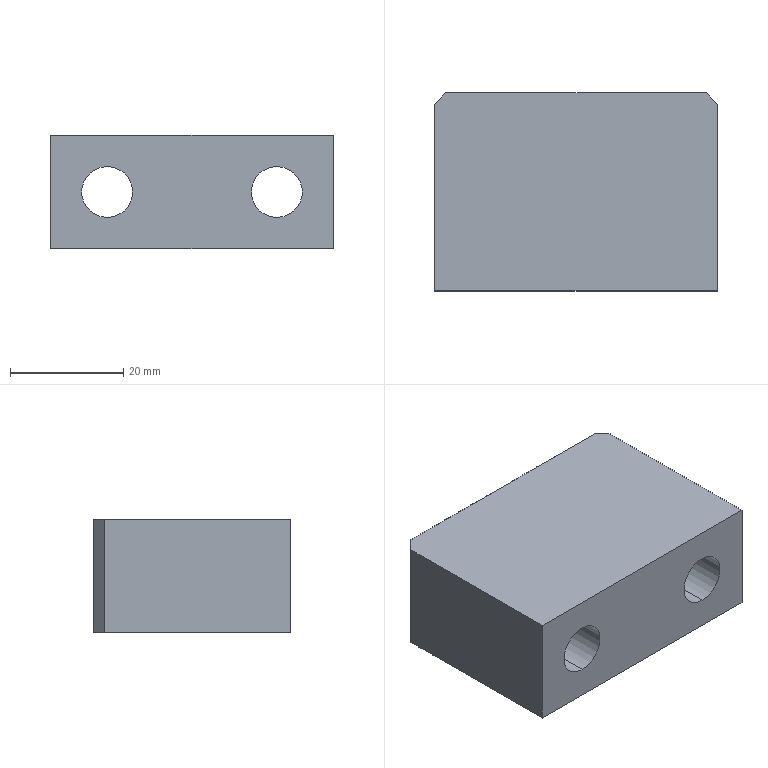Part | SolidWorks | features Chamfer 1, Extrusion 1, HoleWzd 1 | 1 solid | 18 faces | box 50 x 35 x 20 mm | volume 27074 mm3 | plane 10 | cylinder 8 | commonest cylinder face diameters 9 x4 15 x4
STEP:
#1=CARTESIAN_POINT('',(15.,2.5,-7.5));
#2=VERTEX_POINT('',#1);
#3=CARTESIAN_POINT('',(15.,2.5,7.5));
#4=VERTEX_POINT('',#3);
#5=CARTESIAN_POINT('',(15.,2.5,0.));
#6=DIRECTION('',(0.,1.,0.));
#7=DIRECTION('',(0.,0.,1.));
#8=AXIS2_PLACEMENT_3D('',#5,#6,#7);
#9=CIRCLE('',#8,7.5);
#10=EDGE_CURVE('',#2,#4,#9,.T.);
#11=ORIENTED_EDGE('',*,*,#10,.F.);
#12=CARTESIAN_POINT('',(15.,17.5,-7.5));
#13=VERTEX_POINT('',#12);
#14=CARTESIAN_POINT('',(15.,17.5,-7.5));
#15=DIRECTION('',(0.,1.,0.));
#16=VECTOR('',#15,1000.);
#17=LINE('',#14,#16);
#18=EDGE_CURVE('',#2,#13,#17,.T.);
#19=ORIENTED_EDGE('',*,*,#18,.T.);
#20=CARTESIAN_POINT('',(15.,17.5,7.5));
#21=VERTEX_POINT('',#20);
#22=CARTESIAN_POINT('',(15.,17.5,0.));
#23=DIRECTION('',(0.,1.,0.));
#24=DIRECTION('',(0.,0.,1.));
#25=AXIS2_PLACEMENT_3D('',#22,#23,#24);
#26=CIRCLE('',#25,7.5);
#27=EDGE_CURVE('',#13,#21,#26,.T.);
#28=ORIENTED_EDGE('',*,*,#27,.T.);
#29=CARTESIAN_POINT('',(15.,17.5,7.5));
#30=DIRECTION('',(0.,1.,0.));
#31=VECTOR('',#30,1000.);
#32=LINE('',#29,#31);
#33=EDGE_CURVE('',#4,#21,#32,.T.);
#34=ORIENTED_EDGE('',*,*,#33,.F.);
#35=EDGE_LOOP('',(#11,#19,#28,#34));
#36=FACE_OUTER_BOUND('',#35,.T.);
#37=CARTESIAN_POINT('',(15.,17.5,0.));
#38=DIRECTION('',(0.,1.,0.));
#39=DIRECTION('',(0.,0.,1.));
#40=AXIS2_PLACEMENT_3D('',#37,#38,#39);
#41=CYLINDRICAL_SURFACE('',#40,7.5);
#42=ADVANCED_FACE('',(#36),#41,.F.);
#43=CARTESIAN_POINT('',(15.,-17.5,-4.5));
#44=VERTEX_POINT('',#43);
#45=CARTESIAN_POINT('',(15.,-17.5,4.5));
#46=VERTEX_POINT('',#45);
#47=CARTESIAN_POINT('',(15.,-17.5,0.));
#48=DIRECTION('',(0.,1.,0.));
#49=DIRECTION('',(0.,0.,1.));
#50=AXIS2_PLACEMENT_3D('',#47,#48,#49);
#51=CIRCLE('',#50,4.5);
#52=EDGE_CURVE('',#44,#46,#51,.T.);
#53=ORIENTED_EDGE('',*,*,#52,.F.);
#54=CARTESIAN_POINT('',(15.,2.5,-4.5));
#55=VERTEX_POINT('',#54);
#56=CARTESIAN_POINT('',(15.,17.5,-4.5));
#57=DIRECTION('',(0.,1.,0.));
#58=VECTOR('',#57,1000.);
#59=LINE('',#56,#58);
#60=EDGE_CURVE('',#44,#55,#59,.T.);
#61=ORIENTED_EDGE('',*,*,#60,.T.);
#62=CARTESIAN_POINT('',(15.,2.5,4.5));
#63=VERTEX_POINT('',#62);
#64=CARTESIAN_POINT('',(15.,2.5,0.));
#65=DIRECTION('',(0.,1.,0.));
#66=DIRECTION('',(0.,0.,1.));
#67=AXIS2_PLACEMENT_3D('',#64,#65,#66);
#68=CIRCLE('',#67,4.5);
#69=EDGE_CURVE('',#55,#63,#68,.T.);
#70=ORIENTED_EDGE('',*,*,#69,.T.);
#71=CARTESIAN_POINT('',(15.,17.5,4.5));
#72=DIRECTION('',(0.,1.,0.));
#73=VECTOR('',#72,1000.);
#74=LINE('',#71,#73);
#75=EDGE_CURVE('',#46,#63,#74,.T.);
#76=ORIENTED_EDGE('',*,*,#75,.F.);
#77=EDGE_LOOP('',(#53,#61,#70,#76));
#78=FACE_OUTER_BOUND('',#77,.T.);
#79=CARTESIAN_POINT('',(15.,17.5,0.));
#80=DIRECTION('',(0.,1.,0.));
#81=DIRECTION('',(0.,0.,1.));
#82=AXIS2_PLACEMENT_3D('',#79,#80,#81);
#83=CYLINDRICAL_SURFACE('',#82,4.5);
#84=ADVANCED_FACE('',(#78),#83,.F.);
#85=CARTESIAN_POINT('',(-15.,2.5,-7.5));
#86=VERTEX_POINT('',#85);
#87=CARTESIAN_POINT('',(-15.,2.5,7.5));
#88=VERTEX_POINT('',#87);
#89=CARTESIAN_POINT('',(-15.,2.5,0.));
#90=DIRECTION('',(0.,1.,0.));
#91=DIRECTION('',(0.,0.,1.));
#92=AXIS2_PLACEMENT_3D('',#89,#90,#91);
#93=CIRCLE('',#92,7.5);
#94=EDGE_CURVE('',#86,#88,#93,.T.);
#95=ORIENTED_EDGE('',*,*,#94,.F.);
#96=CARTESIAN_POINT('',(-15.,17.5,-7.5));
#97=VERTEX_POINT('',#96);
#98=CARTESIAN_POINT('',(-15.,17.5,-7.5));
#99=DIRECTION('',(0.,1.,0.));
#100=VECTOR('',#99,1000.);
#101=LINE('',#98,#100);
#102=EDGE_CURVE('',#86,#97,#101,.T.);
#103=ORIENTED_EDGE('',*,*,#102,.T.);
#104=CARTESIAN_POINT('',(-15.,17.5,7.5));
#105=VERTEX_POINT('',#104);
#106=CARTESIAN_POINT('',(-15.,17.5,0.));
#107=DIRECTION('',(0.,1.,0.));
#108=DIRECTION('',(0.,0.,1.));
#109=AXIS2_PLACEMENT_3D('',#106,#107,#108);
#110=CIRCLE('',#109,7.5);
#111=EDGE_CURVE('',#97,#105,#110,.T.);
#112=ORIENTED_EDGE('',*,*,#111,.T.);
#113=CARTESIAN_POINT('',(-15.,17.5,7.5));
#114=DIRECTION('',(0.,1.,0.));
#115=VECTOR('',#114,1000.);
#116=LINE('',#113,#115);
#117=EDGE_CURVE('',#88,#105,#116,.T.);
#118=ORIENTED_EDGE('',*,*,#117,.F.);
#119=EDGE_LOOP('',(#95,#103,#112,#118));
#120=FACE_OUTER_BOUND('',#119,.T.);
#121=CARTESIAN_POINT('',(-15.,17.5,0.));
#122=DIRECTION('',(0.,1.,0.));
#123=DIRECTION('',(0.,0.,1.));
#124=AXIS2_PLACEMENT_3D('',#121,#122,#123);
#125=CYLINDRICAL_SURFACE('',#124,7.5);
#126=ADVANCED_FACE('',(#120),#125,.F.);
#127=CARTESIAN_POINT('',(-15.,-17.5,-4.5));
#128=VERTEX_POINT('',#127);
#129=CARTESIAN_POINT('',(-15.,-17.5,4.5));
#130=VERTEX_POINT('',#129);
#131=CARTESIAN_POINT('',(-15.,-17.5,0.));
#132=DIRECTION('',(0.,1.,0.));
#133=DIRECTION('',(0.,0.,1.));
#134=AXIS2_PLACEMENT_3D('',#131,#132,#133);
#135=CIRCLE('',#134,4.5);
#136=EDGE_CURVE('',#128,#130,#135,.T.);
#137=ORIENTED_EDGE('',*,*,#136,.F.);
#138=CARTESIAN_POINT('',(-15.,2.5,-4.5));
#139=VERTEX_POINT('',#138);
#140=CARTESIAN_POINT('',(-15.,17.5,-4.5));
#141=DIRECTION('',(0.,1.,0.));
#142=VECTOR('',#141,1000.);
#143=LINE('',#140,#142);
#144=EDGE_CURVE('',#128,#139,#143,.T.);
#145=ORIENTED_EDGE('',*,*,#144,.T.);
#146=CARTESIAN_POINT('',(-15.,2.5,4.5));
#147=VERTEX_POINT('',#146);
#148=CARTESIAN_POINT('',(-15.,2.5,0.));
#149=DIRECTION('',(0.,1.,0.));
#150=DIRECTION('',(0.,0.,1.));
#151=AXIS2_PLACEMENT_3D('',#148,#149,#150);
#152=CIRCLE('',#151,4.5);
#153=EDGE_CURVE('',#139,#147,#152,.T.);
#154=ORIENTED_EDGE('',*,*,#153,.T.);
#155=CARTESIAN_POINT('',(-15.,17.5,4.5));
#156=DIRECTION('',(0.,1.,0.));
#157=VECTOR('',#156,1000.);
#158=LINE('',#155,#157);
#159=EDGE_CURVE('',#130,#147,#158,.T.);
#160=ORIENTED_EDGE('',*,*,#159,.F.);
#161=EDGE_LOOP('',(#137,#145,#154,#160));
#162=FACE_OUTER_BOUND('',#161,.T.);
#163=CARTESIAN_POINT('',(-15.,17.5,0.));
#164=DIRECTION('',(0.,1.,0.));
#165=DIRECTION('',(0.,0.,1.));
#166=AXIS2_PLACEMENT_3D('',#163,#164,#165);
#167=CYLINDRICAL_SURFACE('',#166,4.5);
#168=ADVANCED_FACE('',(#162),#167,.F.);
#169=CARTESIAN_POINT('',(25.,-17.5,-10.));
#170=VERTEX_POINT('',#169);
#171=CARTESIAN_POINT('',(25.,15.5,-10.));
#172=VERTEX_POINT('',#171);
#173=CARTESIAN_POINT('',(25.,17.5,-10.));
#174=DIRECTION('',(0.,1.,0.));
#175=VECTOR('',#174,1000.);
#176=LINE('',#173,#175);
#177=EDGE_CURVE('',#170,#172,#176,.T.);
#178=ORIENTED_EDGE('',*,*,#177,.T.);
#179=CARTESIAN_POINT('',(25.,15.5,10.));
#180=VERTEX_POINT('',#179);
#181=CARTESIAN_POINT('',(25.,15.5,10.));
#182=DIRECTION('',(0.,0.,1.));
#183=VECTOR('',#182,1000.);
#184=LINE('',#181,#183);
#185=EDGE_CURVE('',#172,#180,#184,.T.);
#186=ORIENTED_EDGE('',*,*,#185,.T.);
#187=CARTESIAN_POINT('',(25.,-17.5,10.));
#188=VERTEX_POINT('',#187);
#189=CARTESIAN_POINT('',(25.,17.5,10.));
#190=DIRECTION('',(0.,1.,0.));
#191=VECTOR('',#190,1000.);
#192=LINE('',#189,#191);
#193=EDGE_CURVE('',#188,#180,#192,.T.);
#194=ORIENTED_EDGE('',*,*,#193,.F.);
#195=CARTESIAN_POINT('',(25.,-17.5,10.));
#196=DIRECTION('',(0.,0.,-1.));
#197=VECTOR('',#196,1000.);
#198=LINE('',#195,#197);
#199=EDGE_CURVE('',#188,#170,#198,.T.);
#200=ORIENTED_EDGE('',*,*,#199,.T.);
#201=EDGE_LOOP('',(#178,#186,#194,#200));
#202=FACE_OUTER_BOUND('',#201,.T.);
#203=CARTESIAN_POINT('',(25.,17.5,10.));
#204=DIRECTION('',(-1.,0.,0.));
#205=DIRECTION('',(0.,-1.,0.));
#206=AXIS2_PLACEMENT_3D('',#203,#204,#205);
#207=PLANE('',#206);
#208=ADVANCED_FACE('',(#202),#207,.F.);
#209=CARTESIAN_POINT('',(15.,17.5,0.));
#210=DIRECTION('',(0.,1.,0.));
#211=DIRECTION('',(0.,0.,1.));
#212=AXIS2_PLACEMENT_3D('',#209,#210,#211);
#213=CIRCLE('',#212,7.5);
#214=EDGE_CURVE('',#21,#13,#213,.T.);
#215=ORIENTED_EDGE('',*,*,#214,.F.);
#216=ORIENTED_EDGE('',*,*,#27,.F.);
#217=EDGE_LOOP('',(#215,#216));
#218=FACE_BOUND('',#217,.T.);
#219=CARTESIAN_POINT('',(-15.,17.5,0.));
#220=DIRECTION('',(0.,1.,0.));
#221=DIRECTION('',(0.,0.,1.));
#222=AXIS2_PLACEMENT_3D('',#219,#220,#221);
#223=CIRCLE('',#222,7.5);
#224=EDGE_CURVE('',#105,#97,#223,.T.);
#225=ORIENTED_EDGE('',*,*,#224,.F.);
#226=ORIENTED_EDGE('',*,*,#111,.F.);
#227=EDGE_LOOP('',(#225,#226));
#228=FACE_BOUND('',#227,.T.);
#229=CARTESIAN_POINT('',(23.,17.5,10.));
#230=VERTEX_POINT('',#229);
#231=CARTESIAN_POINT('',(-23.,17.5,10.));
#232=VERTEX_POINT('',#231);
#233=CARTESIAN_POINT('',(-25.,17.5,10.));
#234=DIRECTION('',(-1.,0.,0.));
#235=VECTOR('',#234,1000.);
#236=LINE('',#233,#235);
#237=EDGE_CURVE('',#230,#232,#236,.T.);
#238=ORIENTED_EDGE('',*,*,#237,.F.);
#239=CARTESIAN_POINT('',(23.,17.5,-10.));
#240=VERTEX_POINT('',#239);
#241=CARTESIAN_POINT('',(23.,17.5,10.));
#242=DIRECTION('',(0.,0.,-1.));
#243=VECTOR('',#242,1000.);
#244=LINE('',#241,#243);
#245=EDGE_CURVE('',#230,#240,#244,.T.);
#246=ORIENTED_EDGE('',*,*,#245,.T.);
#247=CARTESIAN_POINT('',(-23.,17.5,-10.));
#248=VERTEX_POINT('',#247);
#249=CARTESIAN_POINT('',(-25.,17.5,-10.));
#250=DIRECTION('',(-1.,0.,0.));
#251=VECTOR('',#250,1000.);
#252=LINE('',#249,#251);
#253=EDGE_CURVE('',#240,#248,#252,.T.);
#254=ORIENTED_EDGE('',*,*,#253,.T.);
#255=CARTESIAN_POINT('',(-23.,17.5,10.));
#256=DIRECTION('',(0.,0.,1.));
#257=VECTOR('',#256,1000.);
#258=LINE('',#255,#257);
#259=EDGE_CURVE('',#248,#232,#258,.T.);
#260=ORIENTED_EDGE('',*,*,#259,.T.);
#261=EDGE_LOOP('',(#238,#246,#254,#260));
#262=FACE_OUTER_BOUND('',#261,.T.);
#263=CARTESIAN_POINT('',(-25.,17.5,10.));
#264=DIRECTION('',(0.,-1.,0.));
#265=DIRECTION('',(0.,0.,-1.));
#266=AXIS2_PLACEMENT_3D('',#263,#264,#265);
#267=PLANE('',#266);
#268=ADVANCED_FACE('',(#218,#228,#262),#267,.F.);
#269=CARTESIAN_POINT('',(-25.,15.5,10.));
#270=VERTEX_POINT('',#269);
#271=CARTESIAN_POINT('',(-25.,-17.5,10.));
#272=VERTEX_POINT('',#271);
#273=CARTESIAN_POINT('',(-25.,17.5,10.));
#274=DIRECTION('',(0.,-1.,0.));
#275=VECTOR('',#274,1000.);
#276=LINE('',#273,#275);
#277=EDGE_CURVE('',#270,#272,#276,.T.);
#278=ORIENTED_EDGE('',*,*,#277,.F.);
#279=CARTESIAN_POINT('',(-25.,15.5,-10.));
#280=VERTEX_POINT('',#279);
#281=CARTESIAN_POINT('',(-25.,15.5,10.));
#282=DIRECTION('',(0.,0.,-1.));
#283=VECTOR('',#282,1000.);
#284=LINE('',#281,#283);
#285=EDGE_CURVE('',#270,#280,#284,.T.);
#286=ORIENTED_EDGE('',*,*,#285,.T.);
#287=CARTESIAN_POINT('',(-25.,-17.5,-10.));
#288=VERTEX_POINT('',#287);
#289=CARTESIAN_POINT('',(-25.,17.5,-10.));
#290=DIRECTION('',(0.,-1.,0.));
#291=VECTOR('',#290,1000.);
#292=LINE('',#289,#291);
#293=EDGE_CURVE('',#280,#288,#292,.T.);
#294=ORIENTED_EDGE('',*,*,#293,.T.);
#295=CARTESIAN_POINT('',(-25.,-17.5,10.));
#296=DIRECTION('',(0.,0.,-1.));
#297=VECTOR('',#296,1000.);
#298=LINE('',#295,#297);
#299=EDGE_CURVE('',#272,#288,#298,.T.);
#300=ORIENTED_EDGE('',*,*,#299,.F.);
#301=EDGE_LOOP('',(#278,#286,#294,#300));
#302=FACE_OUTER_BOUND('',#301,.T.);
#303=CARTESIAN_POINT('',(-25.,17.5,10.));
#304=DIRECTION('',(1.,0.,0.));
#305=DIRECTION('',(0.,1.,0.));
#306=AXIS2_PLACEMENT_3D('',#303,#304,#305);
#307=PLANE('',#306);
#308=ADVANCED_FACE('',(#302),#307,.F.);
#309=CARTESIAN_POINT('',(15.,-17.5,0.));
#310=DIRECTION('',(0.,1.,0.));
#311=DIRECTION('',(0.,0.,1.));
#312=AXIS2_PLACEMENT_3D('',#309,#310,#311);
#313=CIRCLE('',#312,4.5);
#314=EDGE_CURVE('',#46,#44,#313,.T.);
#315=ORIENTED_EDGE('',*,*,#314,.T.);
#316=ORIENTED_EDGE('',*,*,#52,.T.);
#317=EDGE_LOOP('',(#315,#316));
#318=FACE_BOUND('',#317,.T.);
#319=CARTESIAN_POINT('',(-15.,-17.5,0.));
#320=DIRECTION('',(0.,1.,0.));
#321=DIRECTION('',(0.,0.,1.));
#322=AXIS2_PLACEMENT_3D('',#319,#320,#321);
#323=CIRCLE('',#322,4.5);
#324=EDGE_CURVE('',#130,#128,#323,.T.);
#325=ORIENTED_EDGE('',*,*,#324,.T.);
#326=ORIENTED_EDGE('',*,*,#136,.T.);
#327=EDGE_LOOP('',(#325,#326));
#328=FACE_BOUND('',#327,.T.);
#329=CARTESIAN_POINT('',(-25.,-17.5,-10.));
#330=DIRECTION('',(1.,0.,0.));
#331=VECTOR('',#330,1000.);
#332=LINE('',#329,#331);
#333=EDGE_CURVE('',#288,#170,#332,.T.);
#334=ORIENTED_EDGE('',*,*,#333,.T.);
#335=ORIENTED_EDGE('',*,*,#199,.F.);
#336=CARTESIAN_POINT('',(-25.,-17.5,10.));
#337=DIRECTION('',(1.,0.,0.));
#338=VECTOR('',#337,1000.);
#339=LINE('',#336,#338);
#340=EDGE_CURVE('',#272,#188,#339,.T.);
#341=ORIENTED_EDGE('',*,*,#340,.F.);
#342=ORIENTED_EDGE('',*,*,#299,.T.);
#343=EDGE_LOOP('',(#334,#335,#341,#342));
#344=FACE_OUTER_BOUND('',#343,.T.);
#345=CARTESIAN_POINT('',(-25.,-17.5,10.));
#346=DIRECTION('',(0.,1.,0.));
#347=DIRECTION('',(0.,0.,1.));
#348=AXIS2_PLACEMENT_3D('',#345,#346,#347);
#349=PLANE('',#348);
#350=ADVANCED_FACE('',(#318,#328,#344),#349,.F.);
#351=ORIENTED_EDGE('',*,*,#193,.T.);
#352=CARTESIAN_POINT('',(20.25,20.25,10.));
#353=DIRECTION('',(-0.7071,0.7071,0.));
#354=VECTOR('',#353,1000.);
#355=LINE('',#352,#354);
#356=EDGE_CURVE('',#180,#230,#355,.T.);
#357=ORIENTED_EDGE('',*,*,#356,.T.);
#358=ORIENTED_EDGE('',*,*,#237,.T.);
#359=CARTESIAN_POINT('',(-20.25,20.25,10.));
#360=DIRECTION('',(-0.7071,-0.7071,0.));
#361=VECTOR('',#360,1000.);
#362=LINE('',#359,#361);
#363=EDGE_CURVE('',#232,#270,#362,.T.);
#364=ORIENTED_EDGE('',*,*,#363,.T.);
#365=ORIENTED_EDGE('',*,*,#277,.T.);
#366=ORIENTED_EDGE('',*,*,#340,.T.);
#367=EDGE_LOOP('',(#351,#357,#358,#364,#365,#366));
#368=FACE_OUTER_BOUND('',#367,.T.);
#369=CARTESIAN_POINT('',(0.,0.,10.));
#370=DIRECTION('',(0.,0.,1.));
#371=DIRECTION('',(1.,0.,0.));
#372=AXIS2_PLACEMENT_3D('',#369,#370,#371);
#373=PLANE('',#372);
#374=ADVANCED_FACE('',(#368),#373,.T.);
#375=ORIENTED_EDGE('',*,*,#253,.F.);
#376=CARTESIAN_POINT('',(23.,17.5,-10.));
#377=DIRECTION('',(0.7071,-0.7071,0.));
#378=VECTOR('',#377,1000.);
#379=LINE('',#376,#378);
#380=EDGE_CURVE('',#240,#172,#379,.T.);
#381=ORIENTED_EDGE('',*,*,#380,.T.);
#382=ORIENTED_EDGE('',*,*,#177,.F.);
#383=ORIENTED_EDGE('',*,*,#333,.F.);
#384=ORIENTED_EDGE('',*,*,#293,.F.);
#385=CARTESIAN_POINT('',(-25.,15.5,-10.));
#386=DIRECTION('',(0.7071,0.7071,0.));
#387=VECTOR('',#386,1000.);
#388=LINE('',#385,#387);
#389=EDGE_CURVE('',#280,#248,#388,.T.);
#390=ORIENTED_EDGE('',*,*,#389,.T.);
#391=EDGE_LOOP('',(#375,#381,#382,#383,#384,#390));
#392=FACE_OUTER_BOUND('',#391,.T.);
#393=CARTESIAN_POINT('',(0.,0.,-10.));
#394=DIRECTION('',(0.,0.,1.));
#395=DIRECTION('',(1.,0.,0.));
#396=AXIS2_PLACEMENT_3D('',#393,#394,#395);
#397=PLANE('',#396);
#398=ADVANCED_FACE('',(#392),#397,.F.);
#399=ORIENTED_EDGE('',*,*,#144,.F.);
#400=ORIENTED_EDGE('',*,*,#324,.F.);
#401=ORIENTED_EDGE('',*,*,#159,.T.);
#402=CARTESIAN_POINT('',(-15.,2.5,0.));
#403=DIRECTION('',(0.,1.,0.));
#404=DIRECTION('',(0.,0.,1.));
#405=AXIS2_PLACEMENT_3D('',#402,#403,#404);
#406=CIRCLE('',#405,4.5);
#407=EDGE_CURVE('',#147,#139,#406,.T.);
#408=ORIENTED_EDGE('',*,*,#407,.T.);
#409=EDGE_LOOP('',(#399,#400,#401,#408));
#410=FACE_OUTER_BOUND('',#409,.T.);
#411=CARTESIAN_POINT('',(-15.,17.5,0.));
#412=DIRECTION('',(0.,1.,0.));
#413=DIRECTION('',(0.,0.,1.));
#414=AXIS2_PLACEMENT_3D('',#411,#412,#413);
#415=CYLINDRICAL_SURFACE('',#414,4.5);
#416=ADVANCED_FACE('',(#410),#415,.F.);
#417=ORIENTED_EDGE('',*,*,#407,.F.);
#418=ORIENTED_EDGE('',*,*,#153,.F.);
#419=EDGE_LOOP('',(#417,#418));
#420=FACE_BOUND('',#419,.T.);
#421=CARTESIAN_POINT('',(-15.,2.5,0.));
#422=DIRECTION('',(0.,1.,0.));
#423=DIRECTION('',(0.,0.,1.));
#424=AXIS2_PLACEMENT_3D('',#421,#422,#423);
#425=CIRCLE('',#424,7.5);
#426=EDGE_CURVE('',#88,#86,#425,.T.);
#427=ORIENTED_EDGE('',*,*,#426,.T.);
#428=ORIENTED_EDGE('',*,*,#94,.T.);
#429=EDGE_LOOP('',(#427,#428));
#430=FACE_OUTER_BOUND('',#429,.T.);
#431=CARTESIAN_POINT('',(-10.5,2.5,0.));
#432=DIRECTION('',(0.,-1.,0.));
#433=DIRECTION('',(0.,0.,-1.));
#434=AXIS2_PLACEMENT_3D('',#431,#432,#433);
#435=PLANE('',#434);
#436=ADVANCED_FACE('',(#420,#430),#435,.F.);
#437=ORIENTED_EDGE('',*,*,#102,.F.);
#438=ORIENTED_EDGE('',*,*,#426,.F.);
#439=ORIENTED_EDGE('',*,*,#117,.T.);
#440=ORIENTED_EDGE('',*,*,#224,.T.);
#441=EDGE_LOOP('',(#437,#438,#439,#440));
#442=FACE_OUTER_BOUND('',#441,.T.);
#443=CARTESIAN_POINT('',(-15.,17.5,0.));
#444=DIRECTION('',(0.,1.,0.));
#445=DIRECTION('',(0.,0.,1.));
#446=AXIS2_PLACEMENT_3D('',#443,#444,#445);
#447=CYLINDRICAL_SURFACE('',#446,7.5);
#448=ADVANCED_FACE('',(#442),#447,.F.);
#449=ORIENTED_EDGE('',*,*,#60,.F.);
#450=ORIENTED_EDGE('',*,*,#314,.F.);
#451=ORIENTED_EDGE('',*,*,#75,.T.);
#452=CARTESIAN_POINT('',(15.,2.5,0.));
#453=DIRECTION('',(0.,1.,0.));
#454=DIRECTION('',(0.,0.,1.));
#455=AXIS2_PLACEMENT_3D('',#452,#453,#454);
#456=CIRCLE('',#455,4.5);
#457=EDGE_CURVE('',#63,#55,#456,.T.);
#458=ORIENTED_EDGE('',*,*,#457,.T.);
#459=EDGE_LOOP('',(#449,#450,#451,#458));
#460=FACE_OUTER_BOUND('',#459,.T.);
#461=CARTESIAN_POINT('',(15.,17.5,0.));
#462=DIRECTION('',(0.,1.,0.));
#463=DIRECTION('',(0.,0.,1.));
#464=AXIS2_PLACEMENT_3D('',#461,#462,#463);
#465=CYLINDRICAL_SURFACE('',#464,4.5);
#466=ADVANCED_FACE('',(#460),#465,.F.);
#467=ORIENTED_EDGE('',*,*,#457,.F.);
#468=ORIENTED_EDGE('',*,*,#69,.F.);
#469=EDGE_LOOP('',(#467,#468));
#470=FACE_BOUND('',#469,.T.);
#471=CARTESIAN_POINT('',(15.,2.5,0.));
#472=DIRECTION('',(0.,1.,0.));
#473=DIRECTION('',(0.,0.,1.));
#474=AXIS2_PLACEMENT_3D('',#471,#472,#473);
#475=CIRCLE('',#474,7.5);
#476=EDGE_CURVE('',#4,#2,#475,.T.);
#477=ORIENTED_EDGE('',*,*,#476,.T.);
#478=ORIENTED_EDGE('',*,*,#10,.T.);
#479=EDGE_LOOP('',(#477,#478));
#480=FACE_OUTER_BOUND('',#479,.T.);
#481=CARTESIAN_POINT('',(19.5,2.5,0.));
#482=DIRECTION('',(0.,-1.,0.));
#483=DIRECTION('',(0.,0.,-1.));
#484=AXIS2_PLACEMENT_3D('',#481,#482,#483);
#485=PLANE('',#484);
#486=ADVANCED_FACE('',(#470,#480),#485,.F.);
#487=ORIENTED_EDGE('',*,*,#18,.F.);
#488=ORIENTED_EDGE('',*,*,#476,.F.);
#489=ORIENTED_EDGE('',*,*,#33,.T.);
#490=ORIENTED_EDGE('',*,*,#214,.T.);
#491=EDGE_LOOP('',(#487,#488,#489,#490));
#492=FACE_OUTER_BOUND('',#491,.T.);
#493=CARTESIAN_POINT('',(15.,17.5,0.));
#494=DIRECTION('',(0.,1.,0.));
#495=DIRECTION('',(0.,0.,1.));
#496=AXIS2_PLACEMENT_3D('',#493,#494,#495);
#497=CYLINDRICAL_SURFACE('',#496,7.5);
#498=ADVANCED_FACE('',(#492),#497,.F.);
#499=ORIENTED_EDGE('',*,*,#356,.F.);
#500=ORIENTED_EDGE('',*,*,#185,.F.);
#501=ORIENTED_EDGE('',*,*,#380,.F.);
#502=ORIENTED_EDGE('',*,*,#245,.F.);
#503=EDGE_LOOP('',(#499,#500,#501,#502));
#504=FACE_OUTER_BOUND('',#503,.T.);
#505=CARTESIAN_POINT('',(23.,17.5,10.));
#506=DIRECTION('',(-0.7071,-0.7071,0.));
#507=DIRECTION('',(0.,0.,-1.));
#508=AXIS2_PLACEMENT_3D('',#505,#506,#507);
#509=PLANE('',#508);
#510=ADVANCED_FACE('',(#504),#509,.F.);
#511=ORIENTED_EDGE('',*,*,#363,.F.);
#512=ORIENTED_EDGE('',*,*,#259,.F.);
#513=ORIENTED_EDGE('',*,*,#389,.F.);
#514=ORIENTED_EDGE('',*,*,#285,.F.);
#515=EDGE_LOOP('',(#511,#512,#513,#514));
#516=FACE_OUTER_BOUND('',#515,.T.);
#517=CARTESIAN_POINT('',(-25.,15.5,10.));
#518=DIRECTION('',(0.7071,-0.7071,0.));
#519=DIRECTION('',(0.,0.,-1.));
#520=AXIS2_PLACEMENT_3D('',#517,#518,#519);
#521=PLANE('',#520);
#522=ADVANCED_FACE('',(#516),#521,.F.);
#523=CLOSED_SHELL('',(#42,#84,#126,#168,#208,#268,#308,#350,#374,#398,#416,#436,#448,#466,#486,#498,#510,#522));
#524=MANIFOLD_SOLID_BREP('',#523);
#525=CARTESIAN_POINT('',(0.,0.,0.));
#526=DIRECTION('',(0.,0.,1.));
#527=DIRECTION('',(1.,0.,0.));
#528=AXIS2_PLACEMENT_3D('',#525,#526,#527);
#529=(LENGTH_UNIT()NAMED_UNIT(*)SI_UNIT(.MILLI.,.METRE.));
#530=UNCERTAINTY_MEASURE_WITH_UNIT(LENGTH_MEASURE(0.00001),#529,'','');
#531=(NAMED_UNIT(*)PLANE_ANGLE_UNIT()SI_UNIT($,.RADIAN.));
#532=(NAMED_UNIT(*)SI_UNIT($,.STERADIAN.)SOLID_ANGLE_UNIT());
#533=(GEOMETRIC_REPRESENTATION_CONTEXT(3)GLOBAL_UNCERTAINTY_ASSIGNED_CONTEXT((#530))GLOBAL_UNIT_ASSIGNED_CONTEXT((#529,#531,#532))REPRESENTATION_CONTEXT('',''));
#534=ADVANCED_BREP_SHAPE_REPRESENTATION('',(#524,#528),#533);